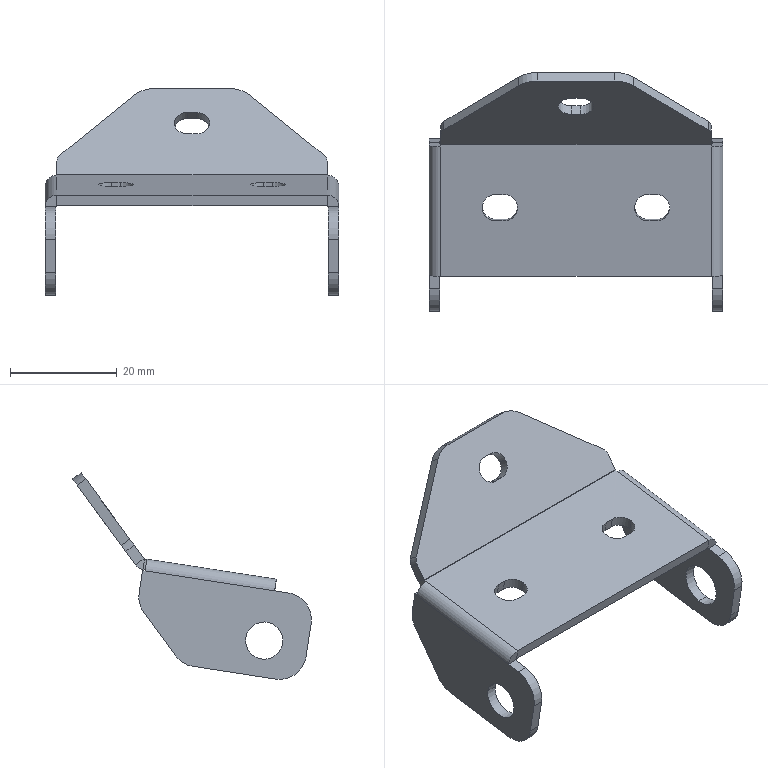Part | SolidWorks | features BaseBody 1 | 1 solid | 71 faces | box 55 x 44.711 x 38.7 mm | volume 5845 mm3 | plane 40 | cylinder 31 | commonest cylinder face diameters 10 x10 5 x9 0.4 x3 4.4 x3 4 x2 7 x2